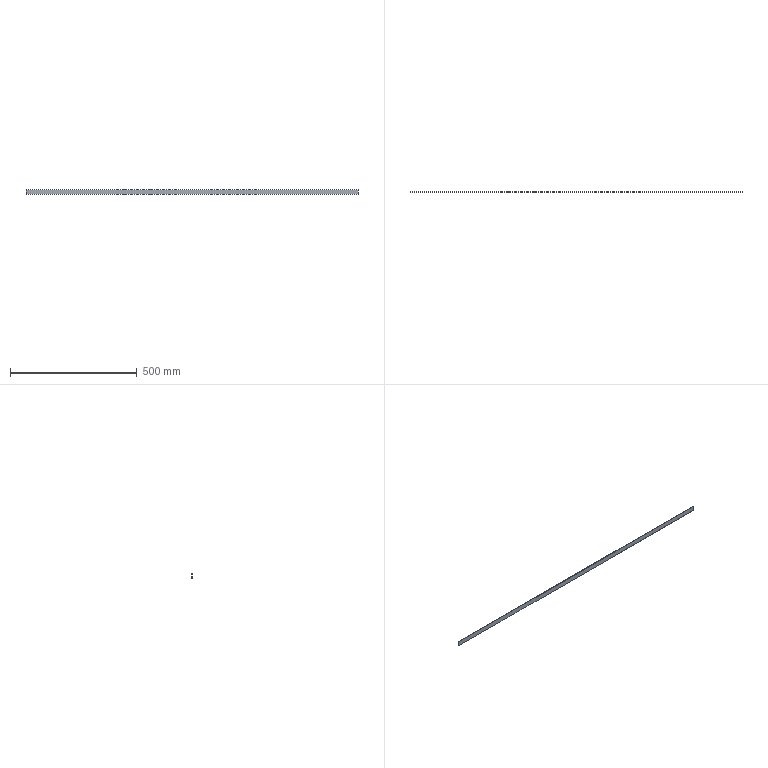Part | NX | features solid 2 | 1 solid | 6 faces | box 1310 x 1.5 x 19.5 mm | volume 38318 mm3 | plane 6
STEP:
#1=CARTESIAN_POINT('',(-273.5,-1497.,1275.));
#2=VERTEX_POINT('',#1);
#3=CARTESIAN_POINT('',(-273.5,-1497.,1294.5));
#4=VERTEX_POINT('',#3);
#5=CARTESIAN_POINT('',(-273.5,-1497.,1275.));
#6=DIRECTION('',(0.,0.,1.));
#7=VECTOR('',#6,1000.);
#8=LINE('',#5,#7);
#9=EDGE_CURVE('',#2,#4,#8,.T.);
#10=ORIENTED_EDGE('',*,*,#9,.T.);
#11=CARTESIAN_POINT('',(1036.5,-1497.,1294.5));
#12=VERTEX_POINT('',#11);
#13=CARTESIAN_POINT('',(-273.5,-1497.,1294.5));
#14=DIRECTION('',(1.,0.,0.));
#15=VECTOR('',#14,1000.);
#16=LINE('',#13,#15);
#17=EDGE_CURVE('',#4,#12,#16,.T.);
#18=ORIENTED_EDGE('',*,*,#17,.T.);
#19=CARTESIAN_POINT('',(1036.5,-1497.,1275.));
#20=VERTEX_POINT('',#19);
#21=CARTESIAN_POINT('',(1036.5,-1497.,1294.5));
#22=DIRECTION('',(0.,0.,-1.));
#23=VECTOR('',#22,1000.);
#24=LINE('',#21,#23);
#25=EDGE_CURVE('',#12,#20,#24,.T.);
#26=ORIENTED_EDGE('',*,*,#25,.T.);
#27=CARTESIAN_POINT('',(1036.5,-1497.,1275.));
#28=DIRECTION('',(-1.,0.,0.));
#29=VECTOR('',#28,1000.);
#30=LINE('',#27,#29);
#31=EDGE_CURVE('',#20,#2,#30,.T.);
#32=ORIENTED_EDGE('',*,*,#31,.T.);
#33=EDGE_LOOP('',(#10,#18,#26,#32));
#34=FACE_BOUND('',#33,.T.);
#35=CARTESIAN_POINT('',(381.5,-1497.,1284.75));
#36=DIRECTION('',(0.,1.,0.));
#37=DIRECTION('',(0.,0.,-1.));
#38=AXIS2_PLACEMENT_3D('',#35,#36,#37);
#39=PLANE('',#38);
#40=ADVANCED_FACE('',(#34),#39,.T.);
#41=CARTESIAN_POINT('',(-273.5,-1498.5,1275.));
#42=VERTEX_POINT('',#41);
#43=CARTESIAN_POINT('',(-273.5,-1498.5,1294.5));
#44=VERTEX_POINT('',#43);
#45=CARTESIAN_POINT('',(-273.5,-1498.5,1275.));
#46=DIRECTION('',(0.,0.,1.));
#47=VECTOR('',#46,1000.);
#48=LINE('',#45,#47);
#49=EDGE_CURVE('',#42,#44,#48,.T.);
#50=ORIENTED_EDGE('',*,*,#49,.F.);
#51=CARTESIAN_POINT('',(1036.5,-1498.5,1275.));
#52=VERTEX_POINT('',#51);
#53=CARTESIAN_POINT('',(1036.5,-1498.5,1275.));
#54=DIRECTION('',(-1.,0.,0.));
#55=VECTOR('',#54,1000.);
#56=LINE('',#53,#55);
#57=EDGE_CURVE('',#52,#42,#56,.T.);
#58=ORIENTED_EDGE('',*,*,#57,.F.);
#59=CARTESIAN_POINT('',(1036.5,-1498.5,1294.5));
#60=VERTEX_POINT('',#59);
#61=CARTESIAN_POINT('',(1036.5,-1498.5,1294.5));
#62=DIRECTION('',(0.,0.,-1.));
#63=VECTOR('',#62,1000.);
#64=LINE('',#61,#63);
#65=EDGE_CURVE('',#60,#52,#64,.T.);
#66=ORIENTED_EDGE('',*,*,#65,.F.);
#67=CARTESIAN_POINT('',(-273.5,-1498.5,1294.5));
#68=DIRECTION('',(1.,0.,0.));
#69=VECTOR('',#68,1000.);
#70=LINE('',#67,#69);
#71=EDGE_CURVE('',#44,#60,#70,.T.);
#72=ORIENTED_EDGE('',*,*,#71,.F.);
#73=EDGE_LOOP('',(#50,#58,#66,#72));
#74=FACE_BOUND('',#73,.T.);
#75=CARTESIAN_POINT('',(381.5,-1498.5,1284.75));
#76=DIRECTION('',(0.,1.,0.));
#77=DIRECTION('',(0.,0.,-1.));
#78=AXIS2_PLACEMENT_3D('',#75,#76,#77);
#79=PLANE('',#78);
#80=ADVANCED_FACE('',(#74),#79,.F.);
#81=ORIENTED_EDGE('',*,*,#31,.F.);
#82=CARTESIAN_POINT('',(1036.5,-1498.5,1275.));
#83=DIRECTION('',(0.,1.,0.));
#84=VECTOR('',#83,1000.);
#85=LINE('',#82,#84);
#86=EDGE_CURVE('',#52,#20,#85,.T.);
#87=ORIENTED_EDGE('',*,*,#86,.F.);
#88=ORIENTED_EDGE('',*,*,#57,.T.);
#89=CARTESIAN_POINT('',(-273.5,-1498.5,1275.));
#90=DIRECTION('',(0.,1.,0.));
#91=VECTOR('',#90,1000.);
#92=LINE('',#89,#91);
#93=EDGE_CURVE('',#42,#2,#92,.T.);
#94=ORIENTED_EDGE('',*,*,#93,.T.);
#95=EDGE_LOOP('',(#81,#87,#88,#94));
#96=FACE_BOUND('',#95,.T.);
#97=CARTESIAN_POINT('',(1036.5,-1498.5,1275.));
#98=DIRECTION('',(0.,0.,-1.));
#99=DIRECTION('',(0.,-1.,0.));
#100=AXIS2_PLACEMENT_3D('',#97,#98,#99);
#101=PLANE('',#100);
#102=ADVANCED_FACE('',(#96),#101,.T.);
#103=ORIENTED_EDGE('',*,*,#25,.F.);
#104=CARTESIAN_POINT('',(1036.5,-1498.5,1294.5));
#105=DIRECTION('',(0.,1.,0.));
#106=VECTOR('',#105,1000.);
#107=LINE('',#104,#106);
#108=EDGE_CURVE('',#60,#12,#107,.T.);
#109=ORIENTED_EDGE('',*,*,#108,.F.);
#110=ORIENTED_EDGE('',*,*,#65,.T.);
#111=ORIENTED_EDGE('',*,*,#86,.T.);
#112=EDGE_LOOP('',(#103,#109,#110,#111));
#113=FACE_BOUND('',#112,.T.);
#114=CARTESIAN_POINT('',(1036.5,-1498.5,1294.5));
#115=DIRECTION('',(1.,0.,0.));
#116=DIRECTION('',(0.,0.,1.));
#117=AXIS2_PLACEMENT_3D('',#114,#115,#116);
#118=PLANE('',#117);
#119=ADVANCED_FACE('',(#113),#118,.T.);
#120=ORIENTED_EDGE('',*,*,#17,.F.);
#121=CARTESIAN_POINT('',(-273.5,-1498.5,1294.5));
#122=DIRECTION('',(0.,1.,0.));
#123=VECTOR('',#122,1000.);
#124=LINE('',#121,#123);
#125=EDGE_CURVE('',#44,#4,#124,.T.);
#126=ORIENTED_EDGE('',*,*,#125,.F.);
#127=ORIENTED_EDGE('',*,*,#71,.T.);
#128=ORIENTED_EDGE('',*,*,#108,.T.);
#129=EDGE_LOOP('',(#120,#126,#127,#128));
#130=FACE_BOUND('',#129,.T.);
#131=CARTESIAN_POINT('',(-273.5,-1498.5,1294.5));
#132=DIRECTION('',(0.,0.,1.));
#133=DIRECTION('',(1.,0.,0.));
#134=AXIS2_PLACEMENT_3D('',#131,#132,#133);
#135=PLANE('',#134);
#136=ADVANCED_FACE('',(#130),#135,.T.);
#137=ORIENTED_EDGE('',*,*,#9,.F.);
#138=ORIENTED_EDGE('',*,*,#93,.F.);
#139=ORIENTED_EDGE('',*,*,#49,.T.);
#140=ORIENTED_EDGE('',*,*,#125,.T.);
#141=EDGE_LOOP('',(#137,#138,#139,#140));
#142=FACE_BOUND('',#141,.T.);
#143=CARTESIAN_POINT('',(-273.5,-1498.5,1275.));
#144=DIRECTION('',(-1.,0.,0.));
#145=DIRECTION('',(0.,0.,1.));
#146=AXIS2_PLACEMENT_3D('',#143,#144,#145);
#147=PLANE('',#146);
#148=ADVANCED_FACE('',(#142),#147,.T.);
#149=CLOSED_SHELL('',(#40,#80,#102,#119,#136,#148));
#150=MANIFOLD_SOLID_BREP('',#149);
#151=(LENGTH_UNIT()NAMED_UNIT(*)SI_UNIT(.MILLI.,.METRE.));
#152=UNCERTAINTY_MEASURE_WITH_UNIT(LENGTH_MEASURE(0.00001),#151,'','');
#153=(NAMED_UNIT(*)PLANE_ANGLE_UNIT()SI_UNIT($,.RADIAN.));
#154=(NAMED_UNIT(*)SI_UNIT($,.STERADIAN.)SOLID_ANGLE_UNIT());
#155=(GEOMETRIC_REPRESENTATION_CONTEXT(3)GLOBAL_UNCERTAINTY_ASSIGNED_CONTEXT((#152))GLOBAL_UNIT_ASSIGNED_CONTEXT((#151,#153,#154))REPRESENTATION_CONTEXT('',''));
#156=ADVANCED_BREP_SHAPE_REPRESENTATION('',(#150),#155);